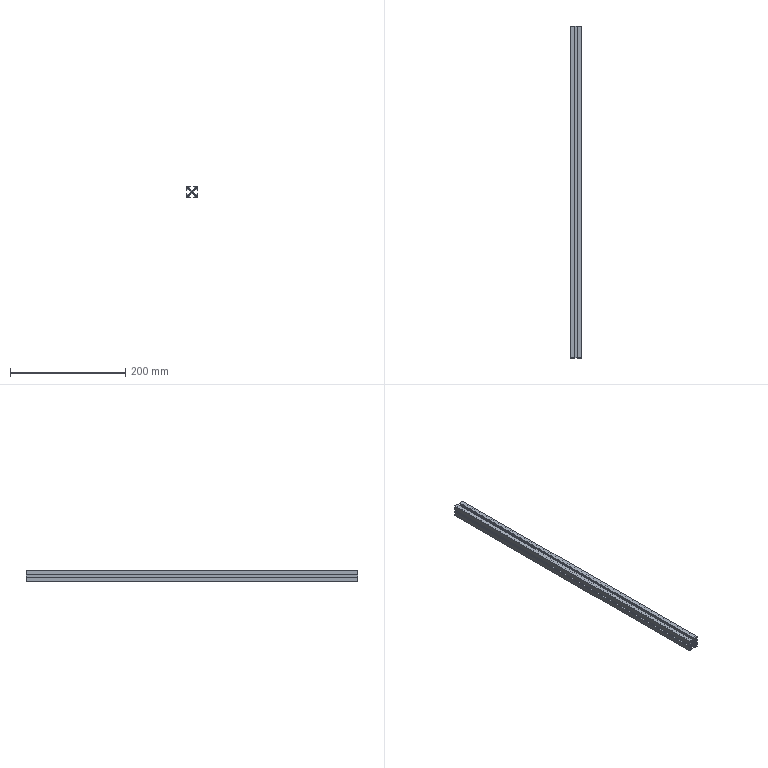Part | STEP file | 20 aluminium profile vertical 1 | 1 solid | 64 faces | box 20 x 575 x 20 mm | volume 102223 mm3 | plane 54 | cylinder 10 | commonest cylinder face diameters 3.3 x10